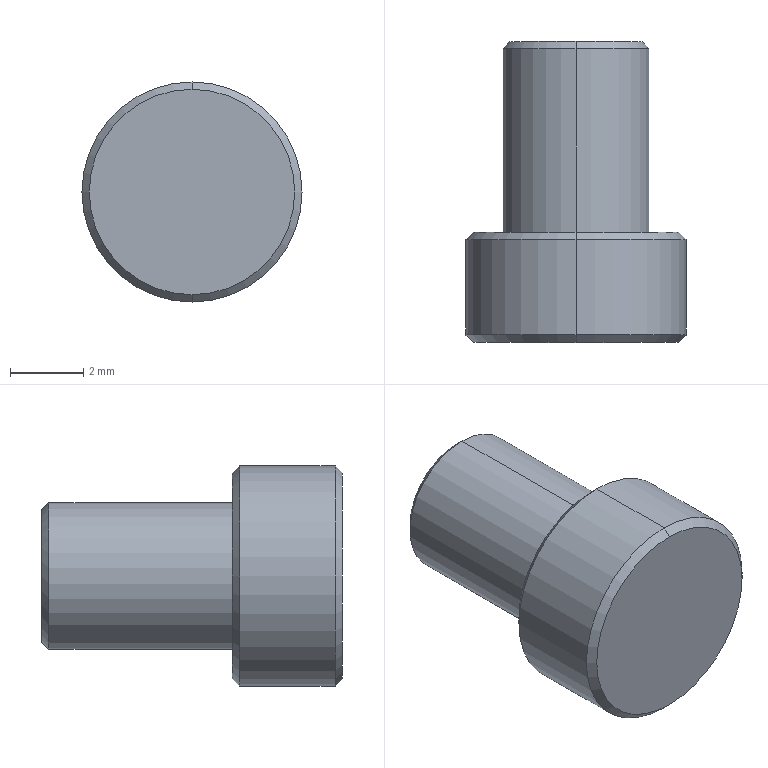Part | SolidWorks | features Chamfer 2, Extrusion 1, HoleWzd 1, ICE 1 | 1 solid | 16 faces | box 6 x 8.2 x 6 mm | volume 132.025 mm3 | cone 6 | cylinder 6 | plane 4 | commonest cylinder face diameters 2.05 x2 4 x2 6 x2
STEP:
#1=CARTESIAN_POINT('',(0.,3.,2.8));
#2=VERTEX_POINT('',#1);
#3=CARTESIAN_POINT('',(0.,3.,-2.8));
#4=VERTEX_POINT('',#3);
#5=CARTESIAN_POINT('',(0.,3.,0.));
#6=DIRECTION('',(0.,1.,0.));
#7=DIRECTION('',(0.,0.,-1.));
#8=AXIS2_PLACEMENT_3D('',#5,#6,#7);
#9=CIRCLE('',#8,2.8);
#10=EDGE_CURVE('',#2,#4,#9,.T.);
#11=ORIENTED_EDGE('',*,*,#10,.F.);
#12=CARTESIAN_POINT('',(0.,2.8,3.));
#13=VERTEX_POINT('',#12);
#14=CARTESIAN_POINT('',(0.,2.8,3.));
#15=DIRECTION('',(0.,-0.7071,0.7071));
#16=VECTOR('',#15,1000.);
#17=LINE('',#14,#16);
#18=EDGE_CURVE('',#2,#13,#17,.T.);
#19=ORIENTED_EDGE('',*,*,#18,.T.);
#20=CARTESIAN_POINT('',(0.,2.8,-3.));
#21=VERTEX_POINT('',#20);
#22=CARTESIAN_POINT('',(0.,2.8,0.));
#23=DIRECTION('',(0.,-1.,0.));
#24=DIRECTION('',(0.,0.,-1.));
#25=AXIS2_PLACEMENT_3D('',#22,#23,#24);
#26=CIRCLE('',#25,3.);
#27=EDGE_CURVE('',#21,#13,#26,.T.);
#28=ORIENTED_EDGE('',*,*,#27,.F.);
#29=CARTESIAN_POINT('',(0.,2.8,-3.));
#30=DIRECTION('',(0.,-0.7071,-0.7071));
#31=VECTOR('',#30,1000.);
#32=LINE('',#29,#31);
#33=EDGE_CURVE('',#4,#21,#32,.T.);
#34=ORIENTED_EDGE('',*,*,#33,.F.);
#35=EDGE_LOOP('',(#11,#19,#28,#34));
#36=FACE_OUTER_BOUND('',#35,.T.);
#37=CARTESIAN_POINT('',(0.,2.8,0.));
#38=DIRECTION('',(0.,-1.,0.));
#39=DIRECTION('',(0.,0.,-1.));
#40=AXIS2_PLACEMENT_3D('',#37,#38,#39);
#41=CONICAL_SURFACE('',#40,3.,0.7854);
#42=ADVANCED_FACE('',(#36),#41,.T.);
#43=CARTESIAN_POINT('',(0.,0.,-2.8));
#44=VERTEX_POINT('',#43);
#45=CARTESIAN_POINT('',(0.,0.,2.8));
#46=VERTEX_POINT('',#45);
#47=CARTESIAN_POINT('',(0.,0.,0.));
#48=DIRECTION('',(0.,-1.,0.));
#49=DIRECTION('',(0.,0.,1.));
#50=AXIS2_PLACEMENT_3D('',#47,#48,#49);
#51=CIRCLE('',#50,2.8);
#52=EDGE_CURVE('',#44,#46,#51,.T.);
#53=ORIENTED_EDGE('',*,*,#52,.F.);
#54=CARTESIAN_POINT('',(0.,0.2,-3.));
#55=VERTEX_POINT('',#54);
#56=CARTESIAN_POINT('',(0.,0.,-2.8));
#57=DIRECTION('',(0.,0.7071,-0.7071));
#58=VECTOR('',#57,1000.);
#59=LINE('',#56,#58);
#60=EDGE_CURVE('',#44,#55,#59,.T.);
#61=ORIENTED_EDGE('',*,*,#60,.T.);
#62=CARTESIAN_POINT('',(0.,0.2,3.));
#63=VERTEX_POINT('',#62);
#64=CARTESIAN_POINT('',(0.,0.2,0.));
#65=DIRECTION('',(0.,1.,0.));
#66=DIRECTION('',(0.,0.,1.));
#67=AXIS2_PLACEMENT_3D('',#64,#65,#66);
#68=CIRCLE('',#67,3.);
#69=EDGE_CURVE('',#63,#55,#68,.T.);
#70=ORIENTED_EDGE('',*,*,#69,.F.);
#71=CARTESIAN_POINT('',(0.,0.,2.8));
#72=DIRECTION('',(0.,0.7071,0.7071));
#73=VECTOR('',#72,1000.);
#74=LINE('',#71,#73);
#75=EDGE_CURVE('',#46,#63,#74,.T.);
#76=ORIENTED_EDGE('',*,*,#75,.F.);
#77=EDGE_LOOP('',(#53,#61,#70,#76));
#78=FACE_OUTER_BOUND('',#77,.T.);
#79=CARTESIAN_POINT('',(0.,0.,0.));
#80=DIRECTION('',(0.,1.,0.));
#81=DIRECTION('',(0.,0.,1.));
#82=AXIS2_PLACEMENT_3D('',#79,#80,#81);
#83=CONICAL_SURFACE('',#82,2.8,0.7854);
#84=ADVANCED_FACE('',(#78),#83,.T.);
#85=CARTESIAN_POINT('',(0.,8.2,1.8));
#86=VERTEX_POINT('',#85);
#87=CARTESIAN_POINT('',(0.,8.2,-1.8));
#88=VERTEX_POINT('',#87);
#89=CARTESIAN_POINT('',(0.,8.2,0.));
#90=DIRECTION('',(0.,1.,0.));
#91=DIRECTION('',(0.,0.,1.));
#92=AXIS2_PLACEMENT_3D('',#89,#90,#91);
#93=CIRCLE('',#92,1.8);
#94=EDGE_CURVE('',#86,#88,#93,.T.);
#95=ORIENTED_EDGE('',*,*,#94,.F.);
#96=CARTESIAN_POINT('',(0.,8.,2.));
#97=VERTEX_POINT('',#96);
#98=CARTESIAN_POINT('',(0.,8.2,1.8));
#99=DIRECTION('',(0.,-0.7071,0.7071));
#100=VECTOR('',#99,1000.);
#101=LINE('',#98,#100);
#102=EDGE_CURVE('',#86,#97,#101,.T.);
#103=ORIENTED_EDGE('',*,*,#102,.T.);
#104=CARTESIAN_POINT('',(0.,8.,-2.));
#105=VERTEX_POINT('',#104);
#106=CARTESIAN_POINT('',(0.,8.,0.));
#107=DIRECTION('',(0.,-1.,0.));
#108=DIRECTION('',(0.,0.,1.));
#109=AXIS2_PLACEMENT_3D('',#106,#107,#108);
#110=CIRCLE('',#109,2.);
#111=EDGE_CURVE('',#105,#97,#110,.T.);
#112=ORIENTED_EDGE('',*,*,#111,.F.);
#113=CARTESIAN_POINT('',(0.,8.2,-1.8));
#114=DIRECTION('',(0.,-0.7071,-0.7071));
#115=VECTOR('',#114,1000.);
#116=LINE('',#113,#115);
#117=EDGE_CURVE('',#88,#105,#116,.T.);
#118=ORIENTED_EDGE('',*,*,#117,.F.);
#119=EDGE_LOOP('',(#95,#103,#112,#118));
#120=FACE_OUTER_BOUND('',#119,.T.);
#121=CARTESIAN_POINT('',(0.,8.2,0.));
#122=DIRECTION('',(0.,-1.,0.));
#123=DIRECTION('',(0.,0.,-1.));
#124=AXIS2_PLACEMENT_3D('',#121,#122,#123);
#125=CONICAL_SURFACE('',#124,1.8,0.7854);
#126=ADVANCED_FACE('',(#120),#125,.T.);
#127=ORIENTED_EDGE('',*,*,#27,.T.);
#128=CARTESIAN_POINT('',(0.,3.,3.));
#129=DIRECTION('',(0.,-1.,0.));
#130=VECTOR('',#129,1000.);
#131=LINE('',#128,#130);
#132=EDGE_CURVE('',#13,#63,#131,.T.);
#133=ORIENTED_EDGE('',*,*,#132,.T.);
#134=ORIENTED_EDGE('',*,*,#69,.T.);
#135=CARTESIAN_POINT('',(0.,3.,-3.));
#136=DIRECTION('',(0.,-1.,0.));
#137=VECTOR('',#136,1000.);
#138=LINE('',#135,#137);
#139=EDGE_CURVE('',#21,#55,#138,.T.);
#140=ORIENTED_EDGE('',*,*,#139,.F.);
#141=EDGE_LOOP('',(#127,#133,#134,#140));
#142=FACE_OUTER_BOUND('',#141,.T.);
#143=CARTESIAN_POINT('',(0.,3.,0.));
#144=DIRECTION('',(0.,-1.,0.));
#145=DIRECTION('',(0.,0.,-1.));
#146=AXIS2_PLACEMENT_3D('',#143,#144,#145);
#147=CYLINDRICAL_SURFACE('',#146,3.);
#148=ADVANCED_FACE('',(#142),#147,.T.);
#149=CARTESIAN_POINT('',(0.,3.,-1.029));
#150=VERTEX_POINT('',#149);
#151=CARTESIAN_POINT('',(0.,3.,1.021));
#152=VERTEX_POINT('',#151);
#153=CARTESIAN_POINT('',(0.,3.,-0.004176));
#154=DIRECTION('',(0.,1.,0.));
#155=DIRECTION('',(0.,0.,-1.));
#156=AXIS2_PLACEMENT_3D('',#153,#154,#155);
#157=CIRCLE('',#156,1.025);
#158=EDGE_CURVE('',#150,#152,#157,.T.);
#159=ORIENTED_EDGE('',*,*,#158,.F.);
#160=CARTESIAN_POINT('',(0.,8.2,-1.029));
#161=VERTEX_POINT('',#160);
#162=CARTESIAN_POINT('',(0.,8.2,-1.029));
#163=DIRECTION('',(0.,1.,0.));
#164=VECTOR('',#163,1000.);
#165=LINE('',#162,#164);
#166=EDGE_CURVE('',#150,#161,#165,.T.);
#167=ORIENTED_EDGE('',*,*,#166,.T.);
#168=CARTESIAN_POINT('',(0.,8.2,1.021));
#169=VERTEX_POINT('',#168);
#170=CARTESIAN_POINT('',(0.,8.2,-0.004176));
#171=DIRECTION('',(0.,1.,0.));
#172=DIRECTION('',(0.,0.,1.));
#173=AXIS2_PLACEMENT_3D('',#170,#171,#172);
#174=CIRCLE('',#173,1.025);
#175=EDGE_CURVE('',#161,#169,#174,.T.);
#176=ORIENTED_EDGE('',*,*,#175,.T.);
#177=CARTESIAN_POINT('',(0.,8.2,1.021));
#178=DIRECTION('',(0.,1.,0.));
#179=VECTOR('',#178,1000.);
#180=LINE('',#177,#179);
#181=EDGE_CURVE('',#152,#169,#180,.T.);
#182=ORIENTED_EDGE('',*,*,#181,.F.);
#183=EDGE_LOOP('',(#159,#167,#176,#182));
#184=FACE_OUTER_BOUND('',#183,.T.);
#185=CARTESIAN_POINT('',(0.,8.2,-0.004176));
#186=DIRECTION('',(0.,1.,0.));
#187=DIRECTION('',(0.,0.,1.));
#188=AXIS2_PLACEMENT_3D('',#185,#186,#187);
#189=CYLINDRICAL_SURFACE('',#188,1.025);
#190=ADVANCED_FACE('',(#184),#189,.F.);
#191=ORIENTED_EDGE('',*,*,#111,.T.);
#192=CARTESIAN_POINT('',(0.,3.,2.));
#193=VERTEX_POINT('',#192);
#194=CARTESIAN_POINT('',(0.,8.2,2.));
#195=DIRECTION('',(0.,-1.,0.));
#196=VECTOR('',#195,1000.);
#197=LINE('',#194,#196);
#198=EDGE_CURVE('',#97,#193,#197,.T.);
#199=ORIENTED_EDGE('',*,*,#198,.T.);
#200=CARTESIAN_POINT('',(0.,3.,-2.));
#201=VERTEX_POINT('',#200);
#202=CARTESIAN_POINT('',(0.,3.,0.));
#203=DIRECTION('',(0.,-1.,0.));
#204=DIRECTION('',(0.,0.,-1.));
#205=AXIS2_PLACEMENT_3D('',#202,#203,#204);
#206=CIRCLE('',#205,2.);
#207=EDGE_CURVE('',#201,#193,#206,.T.);
#208=ORIENTED_EDGE('',*,*,#207,.F.);
#209=CARTESIAN_POINT('',(0.,8.2,-2.));
#210=DIRECTION('',(0.,-1.,0.));
#211=VECTOR('',#210,1000.);
#212=LINE('',#209,#211);
#213=EDGE_CURVE('',#105,#201,#212,.T.);
#214=ORIENTED_EDGE('',*,*,#213,.F.);
#215=EDGE_LOOP('',(#191,#199,#208,#214));
#216=FACE_OUTER_BOUND('',#215,.T.);
#217=CARTESIAN_POINT('',(0.,8.2,0.));
#218=DIRECTION('',(0.,-1.,0.));
#219=DIRECTION('',(0.,0.,-1.));
#220=AXIS2_PLACEMENT_3D('',#217,#218,#219);
#221=CYLINDRICAL_SURFACE('',#220,2.);
#222=ADVANCED_FACE('',(#216),#221,.T.);
#223=ORIENTED_EDGE('',*,*,#198,.F.);
#224=CARTESIAN_POINT('',(0.,8.,0.));
#225=DIRECTION('',(0.,-1.,0.));
#226=DIRECTION('',(0.,0.,1.));
#227=AXIS2_PLACEMENT_3D('',#224,#225,#226);
#228=CIRCLE('',#227,2.);
#229=EDGE_CURVE('',#97,#105,#228,.T.);
#230=ORIENTED_EDGE('',*,*,#229,.T.);
#231=ORIENTED_EDGE('',*,*,#213,.T.);
#232=CARTESIAN_POINT('',(0.,3.,0.));
#233=DIRECTION('',(0.,-1.,0.));
#234=DIRECTION('',(0.,0.,-1.));
#235=AXIS2_PLACEMENT_3D('',#232,#233,#234);
#236=CIRCLE('',#235,2.);
#237=EDGE_CURVE('',#193,#201,#236,.T.);
#238=ORIENTED_EDGE('',*,*,#237,.F.);
#239=EDGE_LOOP('',(#223,#230,#231,#238));
#240=FACE_OUTER_BOUND('',#239,.T.);
#241=CARTESIAN_POINT('',(0.,8.2,0.));
#242=DIRECTION('',(0.,-1.,0.));
#243=DIRECTION('',(0.,0.,-1.));
#244=AXIS2_PLACEMENT_3D('',#241,#242,#243);
#245=CYLINDRICAL_SURFACE('',#244,2.);
#246=ADVANCED_FACE('',(#240),#245,.T.);
#247=ORIENTED_EDGE('',*,*,#166,.F.);
#248=CARTESIAN_POINT('',(0.,3.,-0.004176));
#249=DIRECTION('',(0.,1.,0.));
#250=DIRECTION('',(0.,0.,-1.));
#251=AXIS2_PLACEMENT_3D('',#248,#249,#250);
#252=CIRCLE('',#251,1.025);
#253=EDGE_CURVE('',#152,#150,#252,.T.);
#254=ORIENTED_EDGE('',*,*,#253,.F.);
#255=ORIENTED_EDGE('',*,*,#181,.T.);
#256=CARTESIAN_POINT('',(0.,8.2,-0.004176));
#257=DIRECTION('',(0.,1.,0.));
#258=DIRECTION('',(0.,0.,1.));
#259=AXIS2_PLACEMENT_3D('',#256,#257,#258);
#260=CIRCLE('',#259,1.025);
#261=EDGE_CURVE('',#169,#161,#260,.T.);
#262=ORIENTED_EDGE('',*,*,#261,.T.);
#263=EDGE_LOOP('',(#247,#254,#255,#262));
#264=FACE_OUTER_BOUND('',#263,.T.);
#265=CARTESIAN_POINT('',(0.,8.2,-0.004176));
#266=DIRECTION('',(0.,1.,0.));
#267=DIRECTION('',(0.,0.,1.));
#268=AXIS2_PLACEMENT_3D('',#265,#266,#267);
#269=CYLINDRICAL_SURFACE('',#268,1.025);
#270=ADVANCED_FACE('',(#264),#269,.F.);
#271=CARTESIAN_POINT('',(0.,8.2,0.));
#272=DIRECTION('',(0.,1.,0.));
#273=DIRECTION('',(0.,0.,1.));
#274=AXIS2_PLACEMENT_3D('',#271,#272,#273);
#275=CIRCLE('',#274,1.8);
#276=EDGE_CURVE('',#88,#86,#275,.T.);
#277=ORIENTED_EDGE('',*,*,#276,.T.);
#278=ORIENTED_EDGE('',*,*,#94,.T.);
#279=EDGE_LOOP('',(#277,#278));
#280=FACE_OUTER_BOUND('',#279,.T.);
#281=ORIENTED_EDGE('',*,*,#261,.F.);
#282=ORIENTED_EDGE('',*,*,#175,.F.);
#283=EDGE_LOOP('',(#281,#282));
#284=FACE_BOUND('',#283,.T.);
#285=CARTESIAN_POINT('',(0.,8.2,0.));
#286=DIRECTION('',(0.,1.,0.));
#287=DIRECTION('',(0.,0.,1.));
#288=AXIS2_PLACEMENT_3D('',#285,#286,#287);
#289=PLANE('',#288);
#290=ADVANCED_FACE('',(#280,#284),#289,.T.);
#291=ORIENTED_EDGE('',*,*,#253,.T.);
#292=ORIENTED_EDGE('',*,*,#158,.T.);
#293=EDGE_LOOP('',(#291,#292));
#294=FACE_OUTER_BOUND('',#293,.T.);
#295=CARTESIAN_POINT('',(0.,3.,0.));
#296=DIRECTION('',(0.,-1.,0.));
#297=DIRECTION('',(0.,0.,-1.));
#298=AXIS2_PLACEMENT_3D('',#295,#296,#297);
#299=PLANE('',#298);
#300=ADVANCED_FACE('',(#294),#299,.F.);
#301=CARTESIAN_POINT('',(0.,3.,0.));
#302=DIRECTION('',(0.,1.,0.));
#303=DIRECTION('',(0.,0.,-1.));
#304=AXIS2_PLACEMENT_3D('',#301,#302,#303);
#305=CIRCLE('',#304,2.8);
#306=EDGE_CURVE('',#4,#2,#305,.T.);
#307=ORIENTED_EDGE('',*,*,#306,.T.);
#308=ORIENTED_EDGE('',*,*,#10,.T.);
#309=EDGE_LOOP('',(#307,#308));
#310=FACE_OUTER_BOUND('',#309,.T.);
#311=ORIENTED_EDGE('',*,*,#207,.T.);
#312=ORIENTED_EDGE('',*,*,#237,.T.);
#313=EDGE_LOOP('',(#311,#312));
#314=FACE_BOUND('',#313,.T.);
#315=CARTESIAN_POINT('',(0.,3.,0.));
#316=DIRECTION('',(0.,-1.,0.));
#317=DIRECTION('',(0.,0.,-1.));
#318=AXIS2_PLACEMENT_3D('',#315,#316,#317);
#319=PLANE('',#318);
#320=ADVANCED_FACE('',(#310,#314),#319,.F.);
#321=ORIENTED_EDGE('',*,*,#132,.F.);
#322=CARTESIAN_POINT('',(0.,2.8,0.));
#323=DIRECTION('',(0.,-1.,0.));
#324=DIRECTION('',(0.,0.,-1.));
#325=AXIS2_PLACEMENT_3D('',#322,#323,#324);
#326=CIRCLE('',#325,3.);
#327=EDGE_CURVE('',#13,#21,#326,.T.);
#328=ORIENTED_EDGE('',*,*,#327,.T.);
#329=ORIENTED_EDGE('',*,*,#139,.T.);
#330=CARTESIAN_POINT('',(0.,0.2,0.));
#331=DIRECTION('',(0.,1.,0.));
#332=DIRECTION('',(0.,0.,1.));
#333=AXIS2_PLACEMENT_3D('',#330,#331,#332);
#334=CIRCLE('',#333,3.);
#335=EDGE_CURVE('',#55,#63,#334,.T.);
#336=ORIENTED_EDGE('',*,*,#335,.T.);
#337=EDGE_LOOP('',(#321,#328,#329,#336));
#338=FACE_OUTER_BOUND('',#337,.T.);
#339=CARTESIAN_POINT('',(0.,3.,0.));
#340=DIRECTION('',(0.,-1.,0.));
#341=DIRECTION('',(0.,0.,-1.));
#342=AXIS2_PLACEMENT_3D('',#339,#340,#341);
#343=CYLINDRICAL_SURFACE('',#342,3.);
#344=ADVANCED_FACE('',(#338),#343,.T.);
#345=CARTESIAN_POINT('',(0.,0.,0.));
#346=DIRECTION('',(0.,-1.,0.));
#347=DIRECTION('',(0.,0.,1.));
#348=AXIS2_PLACEMENT_3D('',#345,#346,#347);
#349=CIRCLE('',#348,2.8);
#350=EDGE_CURVE('',#46,#44,#349,.T.);
#351=ORIENTED_EDGE('',*,*,#350,.T.);
#352=ORIENTED_EDGE('',*,*,#52,.T.);
#353=EDGE_LOOP('',(#351,#352));
#354=FACE_OUTER_BOUND('',#353,.T.);
#355=CARTESIAN_POINT('',(0.,0.,0.));
#356=DIRECTION('',(0.,1.,0.));
#357=DIRECTION('',(0.,0.,1.));
#358=AXIS2_PLACEMENT_3D('',#355,#356,#357);
#359=PLANE('',#358);
#360=ADVANCED_FACE('',(#354),#359,.F.);
#361=ORIENTED_EDGE('',*,*,#102,.F.);
#362=ORIENTED_EDGE('',*,*,#276,.F.);
#363=ORIENTED_EDGE('',*,*,#117,.T.);
#364=ORIENTED_EDGE('',*,*,#229,.F.);
#365=EDGE_LOOP('',(#361,#362,#363,#364));
#366=FACE_OUTER_BOUND('',#365,.T.);
#367=CARTESIAN_POINT('',(0.,8.2,0.));
#368=DIRECTION('',(0.,-1.,0.));
#369=DIRECTION('',(0.,0.,-1.));
#370=AXIS2_PLACEMENT_3D('',#367,#368,#369);
#371=CONICAL_SURFACE('',#370,1.8,0.7854);
#372=ADVANCED_FACE('',(#366),#371,.T.);
#373=ORIENTED_EDGE('',*,*,#60,.F.);
#374=ORIENTED_EDGE('',*,*,#350,.F.);
#375=ORIENTED_EDGE('',*,*,#75,.T.);
#376=ORIENTED_EDGE('',*,*,#335,.F.);
#377=EDGE_LOOP('',(#373,#374,#375,#376));
#378=FACE_OUTER_BOUND('',#377,.T.);
#379=CARTESIAN_POINT('',(0.,0.,0.));
#380=DIRECTION('',(0.,1.,0.));
#381=DIRECTION('',(0.,0.,1.));
#382=AXIS2_PLACEMENT_3D('',#379,#380,#381);
#383=CONICAL_SURFACE('',#382,2.8,0.7854);
#384=ADVANCED_FACE('',(#378),#383,.T.);
#385=ORIENTED_EDGE('',*,*,#18,.F.);
#386=ORIENTED_EDGE('',*,*,#306,.F.);
#387=ORIENTED_EDGE('',*,*,#33,.T.);
#388=ORIENTED_EDGE('',*,*,#327,.F.);
#389=EDGE_LOOP('',(#385,#386,#387,#388));
#390=FACE_OUTER_BOUND('',#389,.T.);
#391=CARTESIAN_POINT('',(0.,2.8,0.));
#392=DIRECTION('',(0.,-1.,0.));
#393=DIRECTION('',(0.,0.,-1.));
#394=AXIS2_PLACEMENT_3D('',#391,#392,#393);
#395=CONICAL_SURFACE('',#394,3.,0.7854);
#396=ADVANCED_FACE('',(#390),#395,.T.);
#397=CLOSED_SHELL('',(#42,#84,#126,#148,#190,#222,#246,#270,#290,#300,#320,#344,#360,#372,#384,#396));
#398=MANIFOLD_SOLID_BREP('',#397);
#399=CARTESIAN_POINT('',(0.,0.,0.));
#400=DIRECTION('',(0.,0.,1.));
#401=DIRECTION('',(1.,0.,0.));
#402=AXIS2_PLACEMENT_3D('',#399,#400,#401);
#403=(LENGTH_UNIT()NAMED_UNIT(*)SI_UNIT(.MILLI.,.METRE.));
#404=UNCERTAINTY_MEASURE_WITH_UNIT(LENGTH_MEASURE(0.00001),#403,'','');
#405=(NAMED_UNIT(*)PLANE_ANGLE_UNIT()SI_UNIT($,.RADIAN.));
#406=(NAMED_UNIT(*)SI_UNIT($,.STERADIAN.)SOLID_ANGLE_UNIT());
#407=(GEOMETRIC_REPRESENTATION_CONTEXT(3)GLOBAL_UNCERTAINTY_ASSIGNED_CONTEXT((#404))GLOBAL_UNIT_ASSIGNED_CONTEXT((#403,#405,#406))REPRESENTATION_CONTEXT('',''));
#408=ADVANCED_BREP_SHAPE_REPRESENTATION('',(#398,#402),#407);